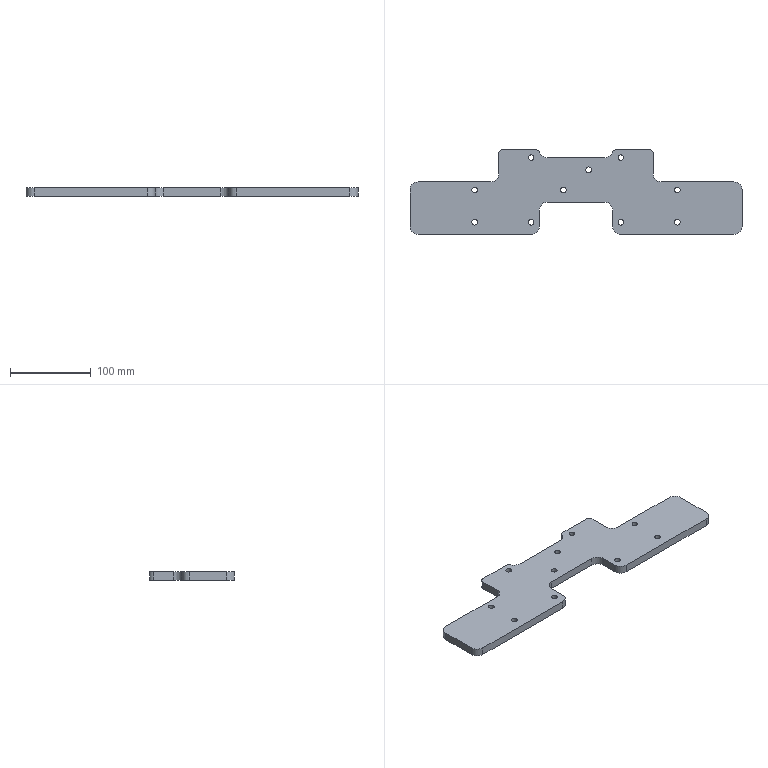Part | STEP file | PE06 | 1 solid | 52 faces | box 411 x 105 x 10 mm | volume 292762 mm3 | cylinder 26 | plane 16 | cone 10 | commonest cylinder face diameters 20 x12 7 x10 10 x4